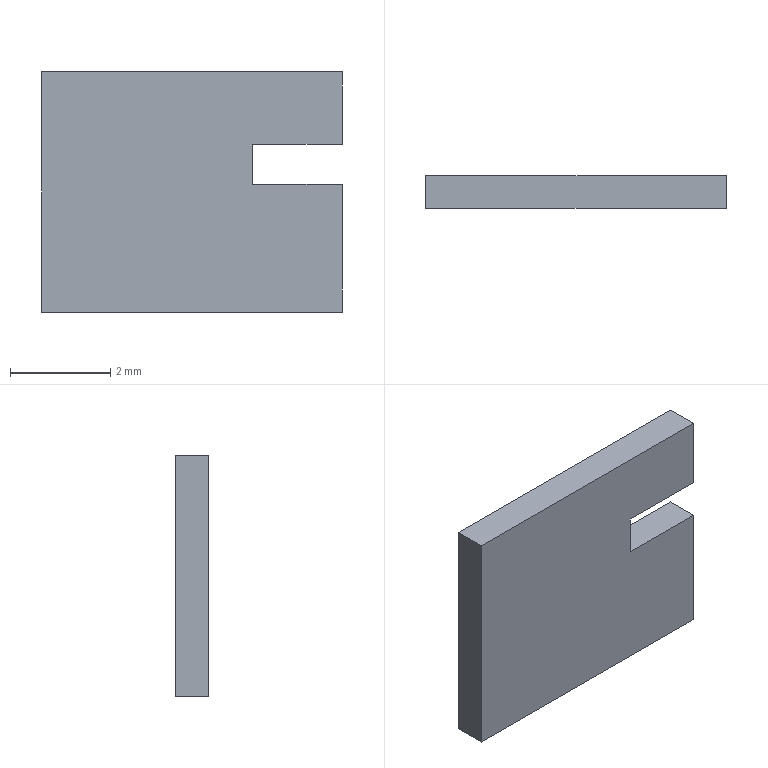Part | STEP file | RJ-USIO-V1_2-220411_130 | 1 solid | 10 faces | box 6 x 0.65 x 4.8 mm | volume 17.792 mm3 | plane 10
STEP:
#1=CARTESIAN_POINT('',(0.,0.,0.));
#2=DIRECTION('',(0.,0.,1.));
#3=DIRECTION('',(1.,0.,0.));
#4=AXIS2_PLACEMENT_3D('',#1,#2,#3);
#5=CARTESIAN_POINT('',(98.15,63.4,4.8));
#6=VERTEX_POINT('',#5);
#7=CARTESIAN_POINT('',(98.15,62.75,4.8));
#8=VERTEX_POINT('',#7);
#9=CARTESIAN_POINT('',(98.15,63.4,4.8));
#10=DIRECTION('',(0.000000012,-1.,0.));
#11=VECTOR('',#10,1.);
#12=LINE('',#9,#11);
#13=CARTESIAN_POINT('',(98.15,63.075,2.4));
#14=DIRECTION('',(1.,0.000000012,0.));
#15=DIRECTION('',(0.000000012,-1.,0.));
#16=AXIS2_PLACEMENT_3D('',#13,#14,#15);
#17=PLANE('',#16);
#18=CARTESIAN_POINT('',(-0.325,-2.4));
#19=DIRECTION('',(1.,0.));
#20=VECTOR('',#19,1.);
#21=LINE('',#18,#20);
#22=(GEOMETRIC_REPRESENTATION_CONTEXT(2)PARAMETRIC_REPRESENTATION_CONTEXT()REPRESENTATION_CONTEXT('',''));
#23=DEFINITIONAL_REPRESENTATION('',(#21),#22);
#24=PCURVE('',#17,#23);
#25=CARTESIAN_POINT('',(101.15,63.075,4.8));
#26=DIRECTION('',(0.,0.,1.));
#27=DIRECTION('',(0.000000012,-1.,0.));
#28=AXIS2_PLACEMENT_3D('',#25,#26,#27);
#29=PLANE('',#28);
#30=CARTESIAN_POINT('',(-0.325,-3.));
#31=DIRECTION('',(1.,0.));
#32=VECTOR('',#31,1.);
#33=LINE('',#30,#32);
#34=(GEOMETRIC_REPRESENTATION_CONTEXT(2)PARAMETRIC_REPRESENTATION_CONTEXT()REPRESENTATION_CONTEXT('',''));
#35=DEFINITIONAL_REPRESENTATION('',(#33),#34);
#36=PCURVE('',#29,#35);
#37=SURFACE_CURVE('',#12,(#24,#36),.PCURVE_S1.);
#38=EDGE_CURVE('',#6,#8,#37,.T.);
#39=ORIENTED_EDGE('',*,*,#38,.T.);
#40=CARTESIAN_POINT('',(98.15,62.75,0.));
#41=VERTEX_POINT('',#40);
#42=CARTESIAN_POINT('',(98.15,62.75,4.8));
#43=DIRECTION('',(0.,0.,-1.));
#44=VECTOR('',#43,1.);
#45=LINE('',#42,#44);
#46=CARTESIAN_POINT('',(0.325,-2.4));
#47=DIRECTION('',(0.,1.));
#48=VECTOR('',#47,1.);
#49=LINE('',#46,#48);
#50=(GEOMETRIC_REPRESENTATION_CONTEXT(2)PARAMETRIC_REPRESENTATION_CONTEXT()REPRESENTATION_CONTEXT('',''));
#51=DEFINITIONAL_REPRESENTATION('',(#49),#50);
#52=PCURVE('',#17,#51);
#53=CARTESIAN_POINT('',(101.15,62.75,2.4));
#54=DIRECTION('',(-0.000000012,1.,0.));
#55=DIRECTION('',(0.,0.,1.));
#56=AXIS2_PLACEMENT_3D('',#53,#54,#55);
#57=PLANE('',#56);
#58=CARTESIAN_POINT('',(2.4,-3.));
#59=DIRECTION('',(-1.,0.));
#60=VECTOR('',#59,1.);
#61=LINE('',#58,#60);
#62=(GEOMETRIC_REPRESENTATION_CONTEXT(2)PARAMETRIC_REPRESENTATION_CONTEXT()REPRESENTATION_CONTEXT('',''));
#63=DEFINITIONAL_REPRESENTATION('',(#61),#62);
#64=PCURVE('',#57,#63);
#65=SURFACE_CURVE('',#45,(#52,#64),.PCURVE_S1.);
#66=EDGE_CURVE('',#8,#41,#65,.T.);
#67=ORIENTED_EDGE('',*,*,#66,.T.);
#68=CARTESIAN_POINT('',(98.15,63.4,0.));
#69=VERTEX_POINT('',#68);
#70=CARTESIAN_POINT('',(98.15,63.4,0.));
#71=DIRECTION('',(0.000000012,-1.,0.));
#72=VECTOR('',#71,1.);
#73=LINE('',#70,#72);
#74=CARTESIAN_POINT('',(-0.325,2.4));
#75=DIRECTION('',(1.,0.));
#76=VECTOR('',#75,1.);
#77=LINE('',#74,#76);
#78=(GEOMETRIC_REPRESENTATION_CONTEXT(2)PARAMETRIC_REPRESENTATION_CONTEXT()REPRESENTATION_CONTEXT('',''));
#79=DEFINITIONAL_REPRESENTATION('',(#77),#78);
#80=PCURVE('',#17,#79);
#81=CARTESIAN_POINT('',(101.15,63.075,0.));
#82=DIRECTION('',(0.,0.,1.));
#83=DIRECTION('',(-0.000000012,1.,0.));
#84=AXIS2_PLACEMENT_3D('',#81,#82,#83);
#85=PLANE('',#84);
#86=CARTESIAN_POINT('',(0.325,3.));
#87=DIRECTION('',(-1.,0.));
#88=VECTOR('',#87,1.);
#89=LINE('',#86,#88);
#90=(GEOMETRIC_REPRESENTATION_CONTEXT(2)PARAMETRIC_REPRESENTATION_CONTEXT()REPRESENTATION_CONTEXT('',''));
#91=DEFINITIONAL_REPRESENTATION('',(#89),#90);
#92=PCURVE('',#85,#91);
#93=SURFACE_CURVE('',#73,(#80,#92),.PCURVE_S1.);
#94=EDGE_CURVE('',#69,#41,#93,.T.);
#95=ORIENTED_EDGE('',*,*,#94,.F.);
#96=CARTESIAN_POINT('',(98.15,63.4,0.));
#97=DIRECTION('',(0.,0.,1.));
#98=VECTOR('',#97,1.);
#99=LINE('',#96,#98);
#100=CARTESIAN_POINT('',(-0.325,2.4));
#101=DIRECTION('',(0.,-1.));
#102=VECTOR('',#101,1.);
#103=LINE('',#100,#102);
#104=(GEOMETRIC_REPRESENTATION_CONTEXT(2)PARAMETRIC_REPRESENTATION_CONTEXT()REPRESENTATION_CONTEXT('',''));
#105=DEFINITIONAL_REPRESENTATION('',(#103),#104);
#106=PCURVE('',#17,#105);
#107=CARTESIAN_POINT('',(101.15,63.4,2.4));
#108=DIRECTION('',(-0.000000012,1.,0.));
#109=DIRECTION('',(0.,0.,1.));
#110=AXIS2_PLACEMENT_3D('',#107,#108,#109);
#111=PLANE('',#110);
#112=CARTESIAN_POINT('',(-2.4,-3.));
#113=DIRECTION('',(1.,0.));
#114=VECTOR('',#113,1.);
#115=LINE('',#112,#114);
#116=(GEOMETRIC_REPRESENTATION_CONTEXT(2)PARAMETRIC_REPRESENTATION_CONTEXT()REPRESENTATION_CONTEXT('',''));
#117=DEFINITIONAL_REPRESENTATION('',(#115),#116);
#118=PCURVE('',#111,#117);
#119=SURFACE_CURVE('',#99,(#106,#118),.PCURVE_S1.);
#120=EDGE_CURVE('',#69,#6,#119,.T.);
#121=ORIENTED_EDGE('',*,*,#120,.T.);
#122=EDGE_LOOP('',(#39,#67,#95,#121));
#123=FACE_BOUND('',#122,.F.);
#124=ADVANCED_FACE('',(#123),#17,.F.);
#125=CARTESIAN_POINT('',(104.15,62.75,4.8));
#126=VERTEX_POINT('',#125);
#127=CARTESIAN_POINT('',(104.15,63.4,4.8));
#128=VERTEX_POINT('',#127);
#129=CARTESIAN_POINT('',(104.15,62.75,4.8));
#130=DIRECTION('',(-0.000000012,1.,0.));
#131=VECTOR('',#130,1.);
#132=LINE('',#129,#131);
#133=CARTESIAN_POINT('',(0.325,3.));
#134=DIRECTION('',(-1.,0.));
#135=VECTOR('',#134,1.);
#136=LINE('',#133,#135);
#137=(GEOMETRIC_REPRESENTATION_CONTEXT(2)PARAMETRIC_REPRESENTATION_CONTEXT()REPRESENTATION_CONTEXT('',''));
#138=DEFINITIONAL_REPRESENTATION('',(#136),#137);
#139=PCURVE('',#29,#138);
#140=CARTESIAN_POINT('',(104.15,63.075,4.075));
#141=DIRECTION('',(1.,0.000000012,0.));
#142=DIRECTION('',(-0.000000012,1.,0.));
#143=AXIS2_PLACEMENT_3D('',#140,#141,#142);
#144=PLANE('',#143);
#145=CARTESIAN_POINT('',(-0.325,0.725));
#146=DIRECTION('',(1.,0.));
#147=VECTOR('',#146,1.);
#148=LINE('',#145,#147);
#149=(GEOMETRIC_REPRESENTATION_CONTEXT(2)PARAMETRIC_REPRESENTATION_CONTEXT()REPRESENTATION_CONTEXT('',''));
#150=DEFINITIONAL_REPRESENTATION('',(#148),#149);
#151=PCURVE('',#144,#150);
#152=SURFACE_CURVE('',#132,(#139,#151),.PCURVE_S1.);
#153=EDGE_CURVE('',#126,#128,#152,.T.);
#154=ORIENTED_EDGE('',*,*,#153,.F.);
#155=CARTESIAN_POINT('',(104.15,62.75,4.8));
#156=DIRECTION('',(-1.,-0.000000012,0.));
#157=VECTOR('',#156,1.);
#158=LINE('',#155,#157);
#159=CARTESIAN_POINT('',(0.325,3.));
#160=DIRECTION('',(0.,-1.));
#161=VECTOR('',#160,1.);
#162=LINE('',#159,#161);
#163=(GEOMETRIC_REPRESENTATION_CONTEXT(2)PARAMETRIC_REPRESENTATION_CONTEXT()REPRESENTATION_CONTEXT('',''));
#164=DEFINITIONAL_REPRESENTATION('',(#162),#163);
#165=PCURVE('',#29,#164);
#166=CARTESIAN_POINT('',(2.4,3.));
#167=DIRECTION('',(0.,-1.));
#168=VECTOR('',#167,1.);
#169=LINE('',#166,#168);
#170=(GEOMETRIC_REPRESENTATION_CONTEXT(2)PARAMETRIC_REPRESENTATION_CONTEXT()REPRESENTATION_CONTEXT('',''));
#171=DEFINITIONAL_REPRESENTATION('',(#169),#170);
#172=PCURVE('',#57,#171);
#173=SURFACE_CURVE('',#158,(#165,#172),.PCURVE_S1.);
#174=EDGE_CURVE('',#126,#8,#173,.T.);
#175=ORIENTED_EDGE('',*,*,#174,.T.);
#176=ORIENTED_EDGE('',*,*,#38,.F.);
#177=CARTESIAN_POINT('',(98.15,63.4,4.8));
#178=DIRECTION('',(1.,0.000000012,0.));
#179=VECTOR('',#178,1.);
#180=LINE('',#177,#179);
#181=CARTESIAN_POINT('',(-0.325,-3.));
#182=DIRECTION('',(0.,1.));
#183=VECTOR('',#182,1.);
#184=LINE('',#181,#183);
#185=(GEOMETRIC_REPRESENTATION_CONTEXT(2)PARAMETRIC_REPRESENTATION_CONTEXT()REPRESENTATION_CONTEXT('',''));
#186=DEFINITIONAL_REPRESENTATION('',(#184),#185);
#187=PCURVE('',#29,#186);
#188=CARTESIAN_POINT('',(2.4,-3.));
#189=DIRECTION('',(0.,1.));
#190=VECTOR('',#189,1.);
#191=LINE('',#188,#190);
#192=(GEOMETRIC_REPRESENTATION_CONTEXT(2)PARAMETRIC_REPRESENTATION_CONTEXT()REPRESENTATION_CONTEXT('',''));
#193=DEFINITIONAL_REPRESENTATION('',(#191),#192);
#194=PCURVE('',#111,#193);
#195=SURFACE_CURVE('',#180,(#187,#194),.PCURVE_S1.);
#196=EDGE_CURVE('',#6,#128,#195,.T.);
#197=ORIENTED_EDGE('',*,*,#196,.T.);
#198=EDGE_LOOP('',(#154,#175,#176,#197));
#199=FACE_BOUND('',#198,.F.);
#200=ADVANCED_FACE('',(#199),#29,.T.);
#201=CARTESIAN_POINT('',(104.15,63.4,3.35));
#202=VERTEX_POINT('',#201);
#203=CARTESIAN_POINT('',(104.15,62.75,3.35));
#204=VERTEX_POINT('',#203);
#205=CARTESIAN_POINT('',(104.15,63.4,3.35));
#206=DIRECTION('',(0.000000012,-1.,0.));
#207=VECTOR('',#206,1.);
#208=LINE('',#205,#207);
#209=CARTESIAN_POINT('',(0.325,-0.725));
#210=DIRECTION('',(-1.,0.));
#211=VECTOR('',#210,1.);
#212=LINE('',#209,#211);
#213=(GEOMETRIC_REPRESENTATION_CONTEXT(2)PARAMETRIC_REPRESENTATION_CONTEXT()REPRESENTATION_CONTEXT('',''));
#214=DEFINITIONAL_REPRESENTATION('',(#212),#213);
#215=PCURVE('',#144,#214);
#216=CARTESIAN_POINT('',(103.257,63.075,3.35));
#217=DIRECTION('',(0.,0.,1.));
#218=DIRECTION('',(-0.000000012,1.,0.));
#219=AXIS2_PLACEMENT_3D('',#216,#217,#218);
#220=PLANE('',#219);
#221=CARTESIAN_POINT('',(0.325,-0.8925));
#222=DIRECTION('',(-1.,0.));
#223=VECTOR('',#222,1.);
#224=LINE('',#221,#223);
#225=(GEOMETRIC_REPRESENTATION_CONTEXT(2)PARAMETRIC_REPRESENTATION_CONTEXT()REPRESENTATION_CONTEXT('',''));
#226=DEFINITIONAL_REPRESENTATION('',(#224),#225);
#227=PCURVE('',#220,#226);
#228=SURFACE_CURVE('',#208,(#215,#227),.PCURVE_S1.);
#229=EDGE_CURVE('',#202,#204,#228,.T.);
#230=ORIENTED_EDGE('',*,*,#229,.T.);
#231=CARTESIAN_POINT('',(104.15,62.75,3.35));
#232=DIRECTION('',(0.,0.,1.));
#233=VECTOR('',#232,1.);
#234=LINE('',#231,#233);
#235=CARTESIAN_POINT('',(-0.325,-0.725));
#236=DIRECTION('',(0.,1.));
#237=VECTOR('',#236,1.);
#238=LINE('',#235,#237);
#239=(GEOMETRIC_REPRESENTATION_CONTEXT(2)PARAMETRIC_REPRESENTATION_CONTEXT()REPRESENTATION_CONTEXT('',''));
#240=DEFINITIONAL_REPRESENTATION('',(#238),#239);
#241=PCURVE('',#144,#240);
#242=CARTESIAN_POINT('',(0.95,3.));
#243=DIRECTION('',(1.,0.));
#244=VECTOR('',#243,1.);
#245=LINE('',#242,#244);
#246=(GEOMETRIC_REPRESENTATION_CONTEXT(2)PARAMETRIC_REPRESENTATION_CONTEXT()REPRESENTATION_CONTEXT('',''));
#247=DEFINITIONAL_REPRESENTATION('',(#245),#246);
#248=PCURVE('',#57,#247);
#249=SURFACE_CURVE('',#234,(#241,#248),.PCURVE_S1.);
#250=EDGE_CURVE('',#204,#126,#249,.T.);
#251=ORIENTED_EDGE('',*,*,#250,.T.);
#252=ORIENTED_EDGE('',*,*,#153,.T.);
#253=CARTESIAN_POINT('',(104.15,63.4,4.8));
#254=DIRECTION('',(0.,0.,-1.));
#255=VECTOR('',#254,1.);
#256=LINE('',#253,#255);
#257=CARTESIAN_POINT('',(0.325,0.725));
#258=DIRECTION('',(0.,-1.));
#259=VECTOR('',#258,1.);
#260=LINE('',#257,#259);
#261=(GEOMETRIC_REPRESENTATION_CONTEXT(2)PARAMETRIC_REPRESENTATION_CONTEXT()REPRESENTATION_CONTEXT('',''));
#262=DEFINITIONAL_REPRESENTATION('',(#260),#261);
#263=PCURVE('',#144,#262);
#264=CARTESIAN_POINT('',(2.4,3.));
#265=DIRECTION('',(-1.,0.));
#266=VECTOR('',#265,1.);
#267=LINE('',#264,#266);
#268=(GEOMETRIC_REPRESENTATION_CONTEXT(2)PARAMETRIC_REPRESENTATION_CONTEXT()REPRESENTATION_CONTEXT('',''));
#269=DEFINITIONAL_REPRESENTATION('',(#267),#268);
#270=PCURVE('',#111,#269);
#271=SURFACE_CURVE('',#256,(#263,#270),.PCURVE_S1.);
#272=EDGE_CURVE('',#128,#202,#271,.T.);
#273=ORIENTED_EDGE('',*,*,#272,.T.);
#274=EDGE_LOOP('',(#230,#251,#252,#273));
#275=FACE_BOUND('',#274,.F.);
#276=ADVANCED_FACE('',(#275),#144,.T.);
#277=CARTESIAN_POINT('',(102.365,63.4,3.35));
#278=VERTEX_POINT('',#277);
#279=CARTESIAN_POINT('',(102.365,62.75,3.35));
#280=VERTEX_POINT('',#279);
#281=CARTESIAN_POINT('',(102.365,63.4,3.35));
#282=DIRECTION('',(0.000000012,-1.,0.));
#283=VECTOR('',#282,1.);
#284=LINE('',#281,#283);
#285=CARTESIAN_POINT('',(0.325,0.8925));
#286=DIRECTION('',(-1.,0.));
#287=VECTOR('',#286,1.);
#288=LINE('',#285,#287);
#289=(GEOMETRIC_REPRESENTATION_CONTEXT(2)PARAMETRIC_REPRESENTATION_CONTEXT()REPRESENTATION_CONTEXT('',''));
#290=DEFINITIONAL_REPRESENTATION('',(#288),#289);
#291=PCURVE('',#220,#290);
#292=CARTESIAN_POINT('',(102.365,63.075,2.95));
#293=DIRECTION('',(1.,0.000000012,0.));
#294=DIRECTION('',(-0.000000012,1.,0.));
#295=AXIS2_PLACEMENT_3D('',#292,#293,#294);
#296=PLANE('',#295);
#297=CARTESIAN_POINT('',(0.325,0.4));
#298=DIRECTION('',(-1.,0.));
#299=VECTOR('',#298,1.);
#300=LINE('',#297,#299);
#301=(GEOMETRIC_REPRESENTATION_CONTEXT(2)PARAMETRIC_REPRESENTATION_CONTEXT()REPRESENTATION_CONTEXT('',''));
#302=DEFINITIONAL_REPRESENTATION('',(#300),#301);
#303=PCURVE('',#296,#302);
#304=SURFACE_CURVE('',#284,(#291,#303),.PCURVE_S1.);
#305=EDGE_CURVE('',#278,#280,#304,.T.);
#306=ORIENTED_EDGE('',*,*,#305,.T.);
#307=CARTESIAN_POINT('',(102.365,62.75,3.35));
#308=DIRECTION('',(1.,0.000000012,0.));
#309=VECTOR('',#308,1.);
#310=LINE('',#307,#309);
#311=CARTESIAN_POINT('',(-0.325,0.8925));
#312=DIRECTION('',(0.,-1.));
#313=VECTOR('',#312,1.);
#314=LINE('',#311,#313);
#315=(GEOMETRIC_REPRESENTATION_CONTEXT(2)PARAMETRIC_REPRESENTATION_CONTEXT()REPRESENTATION_CONTEXT('',''));
#316=DEFINITIONAL_REPRESENTATION('',(#314),#315);
#317=PCURVE('',#220,#316);
#318=CARTESIAN_POINT('',(0.95,1.215));
#319=DIRECTION('',(0.,1.));
#320=VECTOR('',#319,1.);
#321=LINE('',#318,#320);
#322=(GEOMETRIC_REPRESENTATION_CONTEXT(2)PARAMETRIC_REPRESENTATION_CONTEXT()REPRESENTATION_CONTEXT('',''));
#323=DEFINITIONAL_REPRESENTATION('',(#321),#322);
#324=PCURVE('',#57,#323);
#325=SURFACE_CURVE('',#310,(#317,#324),.PCURVE_S1.);
#326=EDGE_CURVE('',#280,#204,#325,.T.);
#327=ORIENTED_EDGE('',*,*,#326,.T.);
#328=ORIENTED_EDGE('',*,*,#229,.F.);
#329=CARTESIAN_POINT('',(104.15,63.4,3.35));
#330=DIRECTION('',(-1.,-0.000000012,0.));
#331=VECTOR('',#330,1.);
#332=LINE('',#329,#331);
#333=CARTESIAN_POINT('',(0.325,-0.8925));
#334=DIRECTION('',(0.,1.));
#335=VECTOR('',#334,1.);
#336=LINE('',#333,#335);
#337=(GEOMETRIC_REPRESENTATION_CONTEXT(2)PARAMETRIC_REPRESENTATION_CONTEXT()REPRESENTATION_CONTEXT('',''));
#338=DEFINITIONAL_REPRESENTATION('',(#336),#337);
#339=PCURVE('',#220,#338);
#340=CARTESIAN_POINT('',(0.95,3.));
#341=DIRECTION('',(0.,-1.));
#342=VECTOR('',#341,1.);
#343=LINE('',#340,#342);
#344=(GEOMETRIC_REPRESENTATION_CONTEXT(2)PARAMETRIC_REPRESENTATION_CONTEXT()REPRESENTATION_CONTEXT('',''));
#345=DEFINITIONAL_REPRESENTATION('',(#343),#344);
#346=PCURVE('',#111,#345);
#347=SURFACE_CURVE('',#332,(#339,#346),.PCURVE_S1.);
#348=EDGE_CURVE('',#202,#278,#347,.T.);
#349=ORIENTED_EDGE('',*,*,#348,.T.);
#350=EDGE_LOOP('',(#306,#327,#328,#349));
#351=FACE_BOUND('',#350,.F.);
#352=ADVANCED_FACE('',(#351),#220,.F.);
#353=CARTESIAN_POINT('',(102.365,63.4,2.55));
#354=VERTEX_POINT('',#353);
#355=CARTESIAN_POINT('',(102.365,62.75,2.55));
#356=VERTEX_POINT('',#355);
#357=CARTESIAN_POINT('',(102.365,63.4,2.55));
#358=DIRECTION('',(0.000000012,-1.,0.));
#359=VECTOR('',#358,1.);
#360=LINE('',#357,#359);
#361=CARTESIAN_POINT('',(0.325,-0.4));
#362=DIRECTION('',(-1.,0.));
#363=VECTOR('',#362,1.);
#364=LINE('',#361,#363);
#365=(GEOMETRIC_REPRESENTATION_CONTEXT(2)PARAMETRIC_REPRESENTATION_CONTEXT()REPRESENTATION_CONTEXT('',''));
#366=DEFINITIONAL_REPRESENTATION('',(#364),#365);
#367=PCURVE('',#296,#366);
#368=CARTESIAN_POINT('',(103.257,63.075,2.55));
#369=DIRECTION('',(0.,0.,1.));
#370=DIRECTION('',(1.,0.000000012,0.));
#371=AXIS2_PLACEMENT_3D('',#368,#369,#370);
#372=PLANE('',#371);
#373=CARTESIAN_POINT('',(-0.8925,0.325));
#374=DIRECTION('',(0.,-1.));
#375=VECTOR('',#374,1.);
#376=LINE('',#373,#375);
#377=(GEOMETRIC_REPRESENTATION_CONTEXT(2)PARAMETRIC_REPRESENTATION_CONTEXT()REPRESENTATION_CONTEXT('',''));
#378=DEFINITIONAL_REPRESENTATION('',(#376),#377);
#379=PCURVE('',#372,#378);
#380=SURFACE_CURVE('',#360,(#367,#379),.PCURVE_S1.);
#381=EDGE_CURVE('',#354,#356,#380,.T.);
#382=ORIENTED_EDGE('',*,*,#381,.T.);
#383=CARTESIAN_POINT('',(102.365,62.75,2.55));
#384=DIRECTION('',(0.,0.,1.));
#385=VECTOR('',#384,1.);
#386=LINE('',#383,#385);
#387=CARTESIAN_POINT('',(-0.325,-0.4));
#388=DIRECTION('',(0.,1.));
#389=VECTOR('',#388,1.);
#390=LINE('',#387,#389);
#391=(GEOMETRIC_REPRESENTATION_CONTEXT(2)PARAMETRIC_REPRESENTATION_CONTEXT()REPRESENTATION_CONTEXT('',''));
#392=DEFINITIONAL_REPRESENTATION('',(#390),#391);
#393=PCURVE('',#296,#392);
#394=CARTESIAN_POINT('',(0.15,1.215));
#395=DIRECTION('',(1.,0.));
#396=VECTOR('',#395,1.);
#397=LINE('',#394,#396);
#398=(GEOMETRIC_REPRESENTATION_CONTEXT(2)PARAMETRIC_REPRESENTATION_CONTEXT()REPRESENTATION_CONTEXT('',''));
#399=DEFINITIONAL_REPRESENTATION('',(#397),#398);
#400=PCURVE('',#57,#399);
#401=SURFACE_CURVE('',#386,(#393,#400),.PCURVE_S1.);
#402=EDGE_CURVE('',#356,#280,#401,.T.);
#403=ORIENTED_EDGE('',*,*,#402,.T.);
#404=ORIENTED_EDGE('',*,*,#305,.F.);
#405=CARTESIAN_POINT('',(102.365,63.4,3.35));
#406=DIRECTION('',(0.,0.,-1.));
#407=VECTOR('',#406,1.);
#408=LINE('',#405,#407);
#409=CARTESIAN_POINT('',(0.325,0.4));
#410=DIRECTION('',(0.,-1.));
#411=VECTOR('',#410,1.);
#412=LINE('',#409,#411);
#413=(GEOMETRIC_REPRESENTATION_CONTEXT(2)PARAMETRIC_REPRESENTATION_CONTEXT()REPRESENTATION_CONTEXT('',''));
#414=DEFINITIONAL_REPRESENTATION('',(#412),#413);
#415=PCURVE('',#296,#414);
#416=CARTESIAN_POINT('',(0.95,1.215));
#417=DIRECTION('',(-1.,0.));
#418=VECTOR('',#417,1.);
#419=LINE('',#416,#418);
#420=(GEOMETRIC_REPRESENTATION_CONTEXT(2)PARAMETRIC_REPRESENTATION_CONTEXT()REPRESENTATION_CONTEXT('',''));
#421=DEFINITIONAL_REPRESENTATION('',(#419),#420);
#422=PCURVE('',#111,#421);
#423=SURFACE_CURVE('',#408,(#415,#422),.PCURVE_S1.);
#424=EDGE_CURVE('',#278,#354,#423,.T.);
#425=ORIENTED_EDGE('',*,*,#424,.T.);
#426=EDGE_LOOP('',(#382,#403,#404,#425));
#427=FACE_BOUND('',#426,.F.);
#428=ADVANCED_FACE('',(#427),#296,.T.);
#429=CARTESIAN_POINT('',(104.15,63.4,2.55));
#430=VERTEX_POINT('',#429);
#431=CARTESIAN_POINT('',(104.15,62.75,2.55));
#432=VERTEX_POINT('',#431);
#433=CARTESIAN_POINT('',(104.15,63.4,2.55));
#434=DIRECTION('',(0.000000012,-1.,0.));
#435=VECTOR('',#434,1.);
#436=LINE('',#433,#435);
#437=CARTESIAN_POINT('',(0.8925,0.325));
#438=DIRECTION('',(0.,-1.));
#439=VECTOR('',#438,1.);
#440=LINE('',#437,#439);
#441=(GEOMETRIC_REPRESENTATION_CONTEXT(2)PARAMETRIC_REPRESENTATION_CONTEXT()REPRESENTATION_CONTEXT('',''));
#442=DEFINITIONAL_REPRESENTATION('',(#440),#441);
#443=PCURVE('',#372,#442);
#444=CARTESIAN_POINT('',(104.15,63.075,1.275));
#445=DIRECTION('',(1.,0.000000012,0.));
#446=DIRECTION('',(-0.000000012,1.,0.));
#447=AXIS2_PLACEMENT_3D('',#444,#445,#446);
#448=PLANE('',#447);
#449=CARTESIAN_POINT('',(0.325,1.275));
#450=DIRECTION('',(-1.,0.));
#451=VECTOR('',#450,1.);
#452=LINE('',#449,#451);
#453=(GEOMETRIC_REPRESENTATION_CONTEXT(2)PARAMETRIC_REPRESENTATION_CONTEXT()REPRESENTATION_CONTEXT('',''));
#454=DEFINITIONAL_REPRESENTATION('',(#452),#453);
#455=PCURVE('',#448,#454);
#456=SURFACE_CURVE('',#436,(#443,#455),.PCURVE_S1.);
#457=EDGE_CURVE('',#430,#432,#456,.T.);
#458=ORIENTED_EDGE('',*,*,#457,.T.);
#459=CARTESIAN_POINT('',(104.15,62.75,2.55));
#460=DIRECTION('',(-1.,-0.000000012,0.));
#461=VECTOR('',#460,1.);
#462=LINE('',#459,#461);
#463=CARTESIAN_POINT('',(0.8925,-0.325));
#464=DIRECTION('',(-1.,0.));
#465=VECTOR('',#464,1.);
#466=LINE('',#463,#465);
#467=(GEOMETRIC_REPRESENTATION_CONTEXT(2)PARAMETRIC_REPRESENTATION_CONTEXT()REPRESENTATION_CONTEXT('',''));
#468=DEFINITIONAL_REPRESENTATION('',(#466),#467);
#469=PCURVE('',#372,#468);
#470=CARTESIAN_POINT('',(0.15,3.));
#471=DIRECTION('',(0.,-1.));
#472=VECTOR('',#471,1.);
#473=LINE('',#470,#472);
#474=(GEOMETRIC_REPRESENTATION_CONTEXT(2)PARAMETRIC_REPRESENTATION_CONTEXT()REPRESENTATION_CONTEXT('',''));
#475=DEFINITIONAL_REPRESENTATION('',(#473),#474);
#476=PCURVE('',#57,#475);
#477=SURFACE_CURVE('',#462,(#469,#476),.PCURVE_S1.);
#478=EDGE_CURVE('',#432,#356,#477,.T.);
#479=ORIENTED_EDGE('',*,*,#478,.T.);
#480=ORIENTED_EDGE('',*,*,#381,.F.);
#481=CARTESIAN_POINT('',(102.365,63.4,2.55));
#482=DIRECTION('',(1.,0.000000012,0.));
#483=VECTOR('',#482,1.);
#484=LINE('',#481,#483);
#485=CARTESIAN_POINT('',(-0.8925,0.325));
#486=DIRECTION('',(1.,0.));
#487=VECTOR('',#486,1.);
#488=LINE('',#485,#487);
#489=(GEOMETRIC_REPRESENTATION_CONTEXT(2)PARAMETRIC_REPRESENTATION_CONTEXT()REPRESENTATION_CONTEXT('',''));
#490=DEFINITIONAL_REPRESENTATION('',(#488),#489);
#491=PCURVE('',#372,#490);
#492=CARTESIAN_POINT('',(0.15,1.215));
#493=DIRECTION('',(0.,1.));
#494=VECTOR('',#493,1.);
#495=LINE('',#492,#494);
#496=(GEOMETRIC_REPRESENTATION_CONTEXT(2)PARAMETRIC_REPRESENTATION_CONTEXT()REPRESENTATION_CONTEXT('',''));
#497=DEFINITIONAL_REPRESENTATION('',(#495),#496);
#498=PCURVE('',#111,#497);
#499=SURFACE_CURVE('',#484,(#491,#498),.PCURVE_S1.);
#500=EDGE_CURVE('',#354,#430,#499,.T.);
#501=ORIENTED_EDGE('',*,*,#500,.T.);
#502=EDGE_LOOP('',(#458,#479,#480,#501));
#503=FACE_BOUND('',#502,.F.);
#504=ADVANCED_FACE('',(#503),#372,.T.);
#505=CARTESIAN_POINT('',(104.15,63.4,0.));
#506=VERTEX_POINT('',#505);
#507=CARTESIAN_POINT('',(104.15,62.75,0.));
#508=VERTEX_POINT('',#507);
#509=CARTESIAN_POINT('',(104.15,63.4,0.));
#510=DIRECTION('',(0.000000012,-1.,0.));
#511=VECTOR('',#510,1.);
#512=LINE('',#509,#511);
#513=CARTESIAN_POINT('',(0.325,-1.275));
#514=DIRECTION('',(-1.,0.));
#515=VECTOR('',#514,1.);
#516=LINE('',#513,#515);
#517=(GEOMETRIC_REPRESENTATION_CONTEXT(2)PARAMETRIC_REPRESENTATION_CONTEXT()REPRESENTATION_CONTEXT('',''));
#518=DEFINITIONAL_REPRESENTATION('',(#516),#517);
#519=PCURVE('',#448,#518);
#520=CARTESIAN_POINT('',(0.325,-3.));
#521=DIRECTION('',(-1.,0.));
#522=VECTOR('',#521,1.);
#523=LINE('',#520,#522);
#524=(GEOMETRIC_REPRESENTATION_CONTEXT(2)PARAMETRIC_REPRESENTATION_CONTEXT()REPRESENTATION_CONTEXT('',''));
#525=DEFINITIONAL_REPRESENTATION('',(#523),#524);
#526=PCURVE('',#85,#525);
#527=SURFACE_CURVE('',#512,(#519,#526),.PCURVE_S1.);
#528=EDGE_CURVE('',#506,#508,#527,.T.);
#529=ORIENTED_EDGE('',*,*,#528,.T.);
#530=CARTESIAN_POINT('',(104.15,62.75,0.));
#531=DIRECTION('',(0.,0.,1.));
#532=VECTOR('',#531,1.);
#533=LINE('',#530,#532);
#534=CARTESIAN_POINT('',(-0.325,-1.275));
#535=DIRECTION('',(0.,1.));
#536=VECTOR('',#535,1.);
#537=LINE('',#534,#536);
#538=(GEOMETRIC_REPRESENTATION_CONTEXT(2)PARAMETRIC_REPRESENTATION_CONTEXT()REPRESENTATION_CONTEXT('',''));
#539=DEFINITIONAL_REPRESENTATION('',(#537),#538);
#540=PCURVE('',#448,#539);
#541=CARTESIAN_POINT('',(-2.4,3.));
#542=DIRECTION('',(1.,0.));
#543=VECTOR('',#542,1.);
#544=LINE('',#541,#543);
#545=(GEOMETRIC_REPRESENTATION_CONTEXT(2)PARAMETRIC_REPRESENTATION_CONTEXT()REPRESENTATION_CONTEXT('',''));
#546=DEFINITIONAL_REPRESENTATION('',(#544),#545);
#547=PCURVE('',#57,#546);
#548=SURFACE_CURVE('',#533,(#540,#547),.PCURVE_S1.);
#549=EDGE_CURVE('',#508,#432,#548,.T.);
#550=ORIENTED_EDGE('',*,*,#549,.T.);
#551=ORIENTED_EDGE('',*,*,#457,.F.);
#552=CARTESIAN_POINT('',(104.15,63.4,2.55));
#553=DIRECTION('',(0.,0.,-1.));
#554=VECTOR('',#553,1.);
#555=LINE('',#552,#554);
#556=CARTESIAN_POINT('',(0.325,1.275));
#557=DIRECTION('',(0.,-1.));
#558=VECTOR('',#557,1.);
#559=LINE('',#556,#558);
#560=(GEOMETRIC_REPRESENTATION_CONTEXT(2)PARAMETRIC_REPRESENTATION_CONTEXT()REPRESENTATION_CONTEXT('',''));
#561=DEFINITIONAL_REPRESENTATION('',(#559),#560);
#562=PCURVE('',#448,#561);
#563=CARTESIAN_POINT('',(0.15,3.));
#564=DIRECTION('',(-1.,0.));
#565=VECTOR('',#564,1.);
#566=LINE('',#563,#565);
#567=(GEOMETRIC_REPRESENTATION_CONTEXT(2)PARAMETRIC_REPRESENTATION_CONTEXT()REPRESENTATION_CONTEXT('',''));
#568=DEFINITIONAL_REPRESENTATION('',(#566),#567);
#569=PCURVE('',#111,#568);
#570=SURFACE_CURVE('',#555,(#562,#569),.PCURVE_S1.);
#571=EDGE_CURVE('',#430,#506,#570,.T.);
#572=ORIENTED_EDGE('',*,*,#571,.T.);
#573=EDGE_LOOP('',(#529,#550,#551,#572));
#574=FACE_BOUND('',#573,.F.);
#575=ADVANCED_FACE('',(#574),#448,.T.);
#576=ORIENTED_EDGE('',*,*,#94,.T.);
#577=CARTESIAN_POINT('',(98.15,62.75,0.));
#578=DIRECTION('',(1.,0.000000012,0.));
#579=VECTOR('',#578,1.);
#580=LINE('',#577,#579);
#581=CARTESIAN_POINT('',(-0.325,3.));
#582=DIRECTION('',(0.,-1.));
#583=VECTOR('',#582,1.);
#584=LINE('',#581,#583);
#585=(GEOMETRIC_REPRESENTATION_CONTEXT(2)PARAMETRIC_REPRESENTATION_CONTEXT()REPRESENTATION_CONTEXT('',''));
#586=DEFINITIONAL_REPRESENTATION('',(#584),#585);
#587=PCURVE('',#85,#586);
#588=CARTESIAN_POINT('',(-2.4,-3.));
#589=DIRECTION('',(0.,1.));
#590=VECTOR('',#589,1.);
#591=LINE('',#588,#590);
#592=(GEOMETRIC_REPRESENTATION_CONTEXT(2)PARAMETRIC_REPRESENTATION_CONTEXT()REPRESENTATION_CONTEXT('',''));
#593=DEFINITIONAL_REPRESENTATION('',(#591),#592);
#594=PCURVE('',#57,#593);
#595=SURFACE_CURVE('',#580,(#587,#594),.PCURVE_S1.);
#596=EDGE_CURVE('',#41,#508,#595,.T.);
#597=ORIENTED_EDGE('',*,*,#596,.T.);
#598=ORIENTED_EDGE('',*,*,#528,.F.);
#599=CARTESIAN_POINT('',(104.15,63.4,0.));
#600=DIRECTION('',(-1.,-0.000000012,0.));
#601=VECTOR('',#600,1.);
#602=LINE('',#599,#601);
#603=CARTESIAN_POINT('',(0.325,-3.));
#604=DIRECTION('',(0.,1.));
#605=VECTOR('',#604,1.);
#606=LINE('',#603,#605);
#607=(GEOMETRIC_REPRESENTATION_CONTEXT(2)PARAMETRIC_REPRESENTATION_CONTEXT()REPRESENTATION_CONTEXT('',''));
#608=DEFINITIONAL_REPRESENTATION('',(#606),#607);
#609=PCURVE('',#85,#608);
#610=CARTESIAN_POINT('',(-2.4,3.));
#611=DIRECTION('',(0.,-1.));
#612=VECTOR('',#611,1.);
#613=LINE('',#610,#612);
#614=(GEOMETRIC_REPRESENTATION_CONTEXT(2)PARAMETRIC_REPRESENTATION_CONTEXT()REPRESENTATION_CONTEXT('',''));
#615=DEFINITIONAL_REPRESENTATION('',(#613),#614);
#616=PCURVE('',#111,#615);
#617=SURFACE_CURVE('',#602,(#609,#616),.PCURVE_S1.);
#618=EDGE_CURVE('',#506,#69,#617,.T.);
#619=ORIENTED_EDGE('',*,*,#618,.T.);
#620=EDGE_LOOP('',(#576,#597,#598,#619));
#621=FACE_BOUND('',#620,.F.);
#622=ADVANCED_FACE('',(#621),#85,.F.);
#623=ORIENTED_EDGE('',*,*,#250,.F.);
#624=ORIENTED_EDGE('',*,*,#326,.F.);
#625=ORIENTED_EDGE('',*,*,#402,.F.);
#626=ORIENTED_EDGE('',*,*,#478,.F.);
#627=ORIENTED_EDGE('',*,*,#549,.F.);
#628=ORIENTED_EDGE('',*,*,#596,.F.);
#629=ORIENTED_EDGE('',*,*,#66,.F.);
#630=ORIENTED_EDGE('',*,*,#174,.F.);
#631=EDGE_LOOP('',(#623,#624,#625,#626,#627,#628,#629,#630));
#632=FACE_BOUND('',#631,.F.);
#633=ADVANCED_FACE('',(#632),#57,.F.);
#634=ORIENTED_EDGE('',*,*,#272,.F.);
#635=ORIENTED_EDGE('',*,*,#196,.F.);
#636=ORIENTED_EDGE('',*,*,#120,.F.);
#637=ORIENTED_EDGE('',*,*,#618,.F.);
#638=ORIENTED_EDGE('',*,*,#571,.F.);
#639=ORIENTED_EDGE('',*,*,#500,.F.);
#640=ORIENTED_EDGE('',*,*,#424,.F.);
#641=ORIENTED_EDGE('',*,*,#348,.F.);
#642=EDGE_LOOP('',(#634,#635,#636,#637,#638,#639,#640,#641));
#643=FACE_BOUND('',#642,.F.);
#644=ADVANCED_FACE('',(#643),#111,.T.);
#645=CLOSED_SHELL('',(#124,#200,#276,#352,#428,#504,#575,#622,#633,#644));
#646=MANIFOLD_SOLID_BREP('',#645);
#647=(LENGTH_UNIT()NAMED_UNIT(*)SI_UNIT(.MILLI.,.METRE.));
#648=UNCERTAINTY_MEASURE_WITH_UNIT(LENGTH_MEASURE(0.0000001),#647,'','');
#649=(NAMED_UNIT(*)PLANE_ANGLE_UNIT()SI_UNIT($,.RADIAN.));
#650=(NAMED_UNIT(*)SI_UNIT($,.STERADIAN.)SOLID_ANGLE_UNIT());
#651=(GEOMETRIC_REPRESENTATION_CONTEXT(3)GLOBAL_UNCERTAINTY_ASSIGNED_CONTEXT((#648))GLOBAL_UNIT_ASSIGNED_CONTEXT((#647,#649,#650))REPRESENTATION_CONTEXT('',''));
#652=ADVANCED_BREP_SHAPE_REPRESENTATION('',(#4,#646),#651);